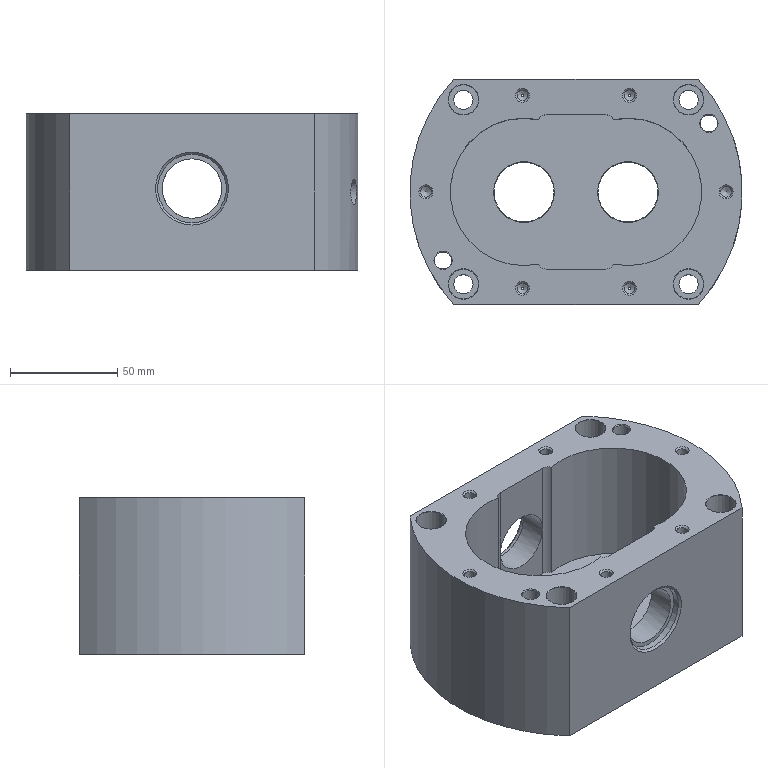NC program | NX | posted with a generic post | part box 155 x 105 x 73.2 mm
Lines 11999 to 12789 of 30727:
(ZLEVEL_PROFILE_COPY_COPY_1 , TOOL : D8)
N23972 T08 M6
N23974 G54
N23976 G17 G0 G90 X-15.89 Y-28.368 B0. C0. S3740 M3
N23978 G43 Z30. H8
N23980 Z-0.1
N23982 G94 G1 X-15.705 Y-29.791 F1000.
N23984 G3 X-15.343 Y-30.362 R0.8
N23986 G2 X-13.894 Y-32. R4. F1600.
N23988 G1 X-10.402
N23990 G3 X-9.789 Y-31.714 R0.8
N23992 G1 X-8.687 Y-30.4
N23994 G0 X-15.89 Y-28.368 Z-0.2
N23996 G1 X-15.705 Y-29.791 F1000.
N23998 G3 X-15.343 Y-30.362 R0.8
N24000 G2 X-13.894 Y-32. R4. F1600.
N24002 G1 X-10.402
N24004 G3 X-9.789 Y-31.714 R0.8
N24006 G1 X-8.687 Y-30.4
N24008 G0 X-15.89 Y-28.368 Z-0.3
N24010 G1 X-15.705 Y-29.791 F1000.
N24012 G3 X-15.343 Y-30.362 R0.8
N24014 G2 X-13.894 Y-32. R4. F1600.
N24016 G1 X-10.402
N24018 G3 X-9.789 Y-31.714 R0.8
N24020 G1 X-8.687 Y-30.4
N24022 G0 X-15.89 Y-28.368 Z-0.4
N24024 G1 X-15.705 Y-29.791 F1000.
N24026 G3 X-15.343 Y-30.362 R0.8
N24028 G2 X-13.894 Y-32. R4. F1600.
N24030 G1 X-10.402
N24032 G3 X-9.789 Y-31.714 R0.8
N24034 G1 X-8.687 Y-30.4
N24036 G0 X-15.89 Y-28.368 Z-0.5
N24038 G1 X-15.705 Y-29.791 F1000.
N24040 G3 X-15.343 Y-30.362 R0.8
N24042 G2 X-13.894 Y-32. R4. F1600.
N24044 G1 X-10.402
N24046 G3 X-9.789 Y-31.714 R0.8
N24048 G1 X-8.687 Y-30.4
N24050 G0 X-15.89 Y-28.368 Z-0.6
N24052 G1 X-15.705 Y-29.791 F1000.
N24054 G3 X-15.343 Y-30.362 R0.8
N24056 G2 X-13.894 Y-32. R4. F1600.
N24058 G1 X-10.402
N24060 G3 X-9.789 Y-31.714 R0.8
N24062 G1 X-8.687 Y-30.4
N24064 G0 X-15.89 Y-28.368 Z-0.7
N24066 G1 X-15.705 Y-29.791 F1000.
N24068 G3 X-15.343 Y-30.362 R0.8
N24070 G2 X-13.894 Y-32. R4. F1600.
N24072 G1 X-10.402
N24074 G3 X-9.789 Y-31.714 R0.8
N24076 G1 X-8.687 Y-30.4
N24078 G0 X-15.89 Y-28.368 Z-0.8
N24080 G1 X-15.705 Y-29.791 F1000.
N24082 G3 X-15.343 Y-30.362 R0.8
N24084 G2 X-13.894 Y-32. R4. F1600.
N24086 G1 X-10.402
N24088 G3 X-9.789 Y-31.714 R0.8
N24090 G1 X-8.687 Y-30.4
N24092 G0 X-15.89 Y-28.368 Z-0.9
N24094 G1 X-15.705 Y-29.791 F1000.
N24096 G3 X-15.343 Y-30.362 R0.8
N24098 G2 X-13.894 Y-32. R4. F1600.
N24100 G1 X-10.402
N24102 G3 X-9.789 Y-31.714 R0.8
N24104 G1 X-8.687 Y-30.4
N24106 G0 X-15.89 Y-28.368 Z-1.
N24108 G1 X-15.705 Y-29.791 F1000.
N24110 G3 X-15.343 Y-30.362 R0.8
N24112 G2 X-13.894 Y-32. R4. F1600.
N24114 G1 X-10.402
N24116 G3 X-9.789 Y-31.714 R0.8
N24118 G1 X-8.687 Y-30.4
N24120 G0 X-15.89 Y-28.368 Z-1.1
N24122 G1 X-15.705 Y-29.791 F1000.
N24124 G3 X-15.343 Y-30.362 R0.8
N24126 G2 X-13.894 Y-32. R4. F1600.
N24128 G1 X-10.402
N24130 G3 X-9.789 Y-31.714 R0.8
N24132 G1 X-8.687 Y-30.4
N24134 G0 X-15.89 Y-28.368 Z-1.2
N24136 G1 X-15.705 Y-29.791 F1000.
N24138 G3 X-15.343 Y-30.362 R0.8
N24140 G2 X-13.894 Y-32. R4. F1600.
N24142 G1 X-10.402
N24144 G3 X-9.789 Y-31.714 R0.8
N24146 G1 X-8.687 Y-30.4
N24148 G0 X-15.89 Y-28.368 Z-1.3
N24150 G1 X-15.705 Y-29.791 F1000.
N24152 G3 X-15.343 Y-30.362 R0.8
N24154 G2 X-13.894 Y-32. R4. F1600.
N24156 G1 X-10.402
N24158 G3 X-9.789 Y-31.714 R0.8
N24160 G1 X-8.687 Y-30.4
N24162 G0 X-15.89 Y-28.368 Z-1.4
N24164 G1 X-15.705 Y-29.791 F1000.
N24166 G3 X-15.343 Y-30.362 R0.8
N24168 G2 X-13.894 Y-32. R4. F1600.
N24170 G1 X-10.402
N24172 G3 X-9.789 Y-31.714 R0.8
N24174 G1 X-8.687 Y-30.4
N24176 G0 X-15.89 Y-28.368 Z-1.5
N24178 G1 X-15.705 Y-29.791 F1000.
N24180 G3 X-15.343 Y-30.362 R0.8
N24182 G2 X-13.894 Y-32. R4. F1600.
N24184 G1 X-10.402
N24186 G3 X-9.789 Y-31.714 R0.8
N24188 G1 X-8.687 Y-30.4
N24190 G0 X-15.89 Y-28.368 Z-1.6
N24192 G1 X-15.705 Y-29.791 F1000.
N24194 G3 X-15.343 Y-30.362 R0.8
N24196 G2 X-13.894 Y-32. R4. F1600.
N24198 G1 X-10.402
N24200 G3 X-9.789 Y-31.714 R0.8
N24202 G1 X-8.687 Y-30.4
N24204 G0 X-15.89 Y-28.368 Z-1.7
N24206 G1 X-15.705 Y-29.791 F1000.
N24208 G3 X-15.343 Y-30.362 R0.8
N24210 G2 X-13.894 Y-32. R4. F1600.
N24212 G1 X-10.402
N24214 G3 X-9.789 Y-31.714 R0.8
N24216 G1 X-8.687 Y-30.4
N24218 G0 X-15.89 Y-28.368 Z-1.8
N24220 G1 X-15.705 Y-29.791 F1000.
N24222 G3 X-15.343 Y-30.362 R0.8
N24224 G2 X-13.894 Y-32. R4. F1600.
N24226 G1 X-10.402
N24228 G3 X-9.789 Y-31.714 R0.8
N24230 G1 X-8.687 Y-30.4
N24232 G0 X-15.89 Y-28.368 Z-1.9
N24234 G1 X-15.705 Y-29.791 F1000.
N24236 G3 X-15.343 Y-30.362 R0.8
N24238 G2 X-13.894 Y-32. R4. F1600.
N24240 G1 X-10.402
N24242 G3 X-9.789 Y-31.714 R0.8
N24244 G1 X-8.687 Y-30.4
N24246 G0 X-15.89 Y-28.368 Z-2.
N24248 G1 X-15.705 Y-29.791 F1000.
N24250 G3 X-15.343 Y-30.362 R0.8
N24252 G2 X-13.894 Y-32. R4. F1600.
N24254 G1 X-10.402
N24256 G3 X-9.789 Y-31.714 R0.8
N24258 G1 X-8.687 Y-30.4
N24260 G0 X-15.89 Y-28.368 Z-2.1
N24262 G1 X-15.705 Y-29.791 F1000.
N24264 G3 X-15.343 Y-30.362 R0.8
N24266 G2 X-13.894 Y-32. R4. F1600.
N24268 G1 X-10.402
N24270 G3 X-9.789 Y-31.714 R0.8
N24272 G1 X-8.687 Y-30.4
N24274 G0 X-15.89 Y-28.368 Z-2.2
N24276 G1 X-15.705 Y-29.791 F1000.
N24278 G3 X-15.343 Y-30.362 R0.8
N24280 G2 X-13.894 Y-32. R4. F1600.
N24282 G1 X-10.402
N24284 G3 X-9.789 Y-31.714 R0.8
N24286 G1 X-8.687 Y-30.4
N24288 G0 X-15.89 Y-28.368 Z-2.3
N24290 G1 X-15.705 Y-29.791 F1000.
N24292 G3 X-15.343 Y-30.362 R0.8
N24294 G2 X-13.894 Y-32. R4. F1600.
N24296 G1 X-10.402
N24298 G3 X-9.789 Y-31.714 R0.8
N24300 G1 X-8.687 Y-30.4
N24302 G0 X-15.89 Y-28.368 Z-2.4
N24304 G1 X-15.705 Y-29.791 F1000.
N24306 G3 X-15.343 Y-30.362 R0.8
N24308 G2 X-13.894 Y-32. R4. F1600.
N24310 G1 X-10.402
N24312 G3 X-9.789 Y-31.714 R0.8
N24314 G1 X-8.687 Y-30.4
N24316 G0 X-15.89 Y-28.368 Z-2.5
N24318 G1 X-15.705 Y-29.791 F1000.
N24320 G3 X-15.343 Y-30.362 R0.8
N24322 G2 X-13.894 Y-32. R4. F1600.
N24324 G1 X-10.402
N24326 G3 X-9.789 Y-31.714 R0.8
N24328 G1 X-8.687 Y-30.4
N24330 G0 X-15.89 Y-28.368 Z-2.6
N24332 G1 X-15.705 Y-29.791 F1000.
N24334 G3 X-15.343 Y-30.362 R0.8
N24336 G2 X-13.894 Y-32. R4. F1600.
N24338 G1 X-10.402
N24340 G3 X-9.789 Y-31.714 R0.8
N24342 G1 X-8.687 Y-30.4
N24344 G0 X-15.89 Y-28.368 Z-2.7
N24346 G1 X-15.705 Y-29.791 F1000.
N24348 G3 X-15.343 Y-30.362 R0.8
N24350 G2 X-13.894 Y-32. R4. F1600.
N24352 G1 X-10.402
N24354 G3 X-9.789 Y-31.714 R0.8
N24356 G1 X-8.687 Y-30.4
N24358 G0 X-15.89 Y-28.368 Z-2.8
N24360 G1 X-15.705 Y-29.791 F1000.
N24362 G3 X-15.343 Y-30.362 R0.8
N24364 G2 X-13.894 Y-32. R4. F1600.
N24366 G1 X-10.402
N24368 G3 X-9.789 Y-31.714 R0.8
N24370 G1 X-8.687 Y-30.4
N24372 G0 X-15.89 Y-28.368 Z-2.9
N24374 G1 X-15.705 Y-29.791 F1000.
N24376 G3 X-15.343 Y-30.362 R0.8
N24378 G2 X-13.894 Y-32. R4. F1600.
N24380 G1 X-10.402
N24382 G3 X-9.789 Y-31.714 R0.8
N24384 G1 X-8.687 Y-30.4
N24386 G0 X-15.89 Y-28.368 Z-3.
N24388 G1 X-15.705 Y-29.791 F1000.
N24390 G3 X-15.343 Y-30.362 R0.8
N24392 G2 X-13.894 Y-32. R4. F1600.
N24394 G1 X-10.402
N24396 G3 X-9.789 Y-31.714 R0.8
N24398 G1 X-8.687 Y-30.4
N24400 G0 X-15.89 Y-28.368 Z-3.1
N24402 G1 X-15.705 Y-29.791 F1000.
N24404 G3 X-15.343 Y-30.362 R0.8
N24406 G2 X-13.894 Y-32. R4. F1600.
N24408 G1 X-10.402
N24410 G3 X-9.789 Y-31.714 R0.8
N24412 G1 X-8.687 Y-30.4
N24414 G0 X-15.89 Y-28.368 Z-3.2
N24416 G1 X-15.705 Y-29.791 F1000.
N24418 G3 X-15.343 Y-30.362 R0.8
N24420 G2 X-13.894 Y-32. R4. F1600.
N24422 G1 X-10.402
N24424 G3 X-9.789 Y-31.714 R0.8
N24426 G1 X-8.687 Y-30.4
N24428 G0 X-15.89 Y-28.368 Z-3.3
N24430 G1 X-15.705 Y-29.791 F1000.
N24432 G3 X-15.343 Y-30.362 R0.8
N24434 G2 X-13.894 Y-32. R4. F1600.
N24436 G1 X-10.402
N24438 G3 X-9.789 Y-31.714 R0.8
N24440 G1 X-8.687 Y-30.4
N24442 G0 X-15.89 Y-28.368 Z-3.4
N24444 G1 X-15.705 Y-29.791 F1000.
N24446 G3 X-15.343 Y-30.362 R0.8
N24448 G2 X-13.894 Y-32. R4. F1600.
N24450 G1 X-10.402
N24452 G3 X-9.789 Y-31.714 R0.8
N24454 G1 X-8.687 Y-30.4
N24456 G0 X-15.89 Y-28.368 Z-3.5
N24458 G1 X-15.705 Y-29.791 F1000.
N24460 G3 X-15.343 Y-30.362 R0.8
N24462 G2 X-13.894 Y-32. R4. F1600.
N24464 G1 X-10.402
N24466 G3 X-9.789 Y-31.714 R0.8
N24468 G1 X-8.687 Y-30.4
N24470 G0 X-15.89 Y-28.368 Z-3.6
N24472 G1 X-15.705 Y-29.791 F1000.
N24474 G3 X-15.343 Y-30.362 R0.8
N24476 G2 X-13.894 Y-32. R4. F1600.
N24478 G1 X-10.402
N24480 G3 X-9.789 Y-31.714 R0.8
N24482 G1 X-8.687 Y-30.4
N24484 G0 X-15.89 Y-28.368 Z-3.7
N24486 G1 X-15.705 Y-29.791 F1000.
N24488 G3 X-15.343 Y-30.362 R0.8
N24490 G2 X-13.894 Y-32. R4. F1600.
N24492 G1 X-10.402
N24494 G3 X-9.789 Y-31.714 R0.8
N24496 G1 X-8.687 Y-30.4
N24498 G0 X-15.89 Y-28.368 Z-3.8
N24500 G1 X-15.705 Y-29.791 F1000.
N24502 G3 X-15.343 Y-30.362 R0.8
N24504 G2 X-13.894 Y-32. R4. F1600.
N24506 G1 X-10.402
N24508 G3 X-9.789 Y-31.714 R0.8
N24510 G1 X-8.687 Y-30.4
N24512 G0 X-15.89 Y-28.368 Z-3.9
N24514 G1 X-15.705 Y-29.791 F1000.
N24516 G3 X-15.343 Y-30.362 R0.8
N24518 G2 X-13.894 Y-32. R4. F1600.
N24520 G1 X-10.402
N24522 G3 X-9.789 Y-31.714 R0.8
N24524 G1 X-8.687 Y-30.4
N24526 G0 X-15.89 Y-28.368 Z-4.
N24528 G1 X-15.705 Y-29.791 F1000.
N24530 G3 X-15.343 Y-30.362 R0.8
N24532 G2 X-13.894 Y-32. R4. F1600.
N24534 G1 X-10.402
N24536 G3 X-9.789 Y-31.714 R0.8
N24538 G1 X-8.687 Y-30.4
N24540 G0 X-15.89 Y-28.368 Z-4.1
N24542 G1 X-15.705 Y-29.791 F1000.
N24544 G3 X-15.343 Y-30.362 R0.8
N24546 G2 X-13.894 Y-32. R4. F1600.
N24548 G1 X-10.402
N24550 G3 X-9.789 Y-31.714 R0.8
N24552 G1 X-8.687 Y-30.4
N24554 G0 X-15.89 Y-28.368 Z-4.2
N24556 G1 X-15.705 Y-29.791 F1000.
N24558 G3 X-15.343 Y-30.362 R0.8
N24560 G2 X-13.894 Y-32. R4. F1600.
N24562 G1 X-10.402
N24564 G3 X-9.789 Y-31.714 R0.8
N24566 G1 X-8.687 Y-30.4
N24568 G0 X-15.89 Y-28.368 Z-4.3
N24570 G1 X-15.705 Y-29.791 F1000.
N24572 G3 X-15.343 Y-30.362 R0.8
N24574 G2 X-13.894 Y-32. R4. F1600.
N24576 G1 X-10.402
N24578 G3 X-9.789 Y-31.714 R0.8
N24580 G1 X-8.687 Y-30.4
N24582 G0 X-15.89 Y-28.368 Z-4.4
N24584 G1 X-15.705 Y-29.791 F1000.
N24586 G3 X-15.343 Y-30.362 R0.8
N24588 G2 X-13.894 Y-32. R4. F1600.
N24590 G1 X-10.402
N24592 G3 X-9.789 Y-31.714 R0.8
N24594 G1 X-8.687 Y-30.4
N24596 G0 X-15.89 Y-28.368 Z-4.5
N24598 G1 X-15.705 Y-29.791 F1000.
N24600 G3 X-15.343 Y-30.362 R0.8
N24602 G2 X-13.894 Y-32. R4. F1600.
N24604 G1 X-10.402
N24606 G3 X-9.789 Y-31.714 R0.8
N24608 G1 X-8.687 Y-30.4
N24610 G0 X-15.89 Y-28.368 Z-4.6
N24612 G1 X-15.705 Y-29.791 F1000.
N24614 G3 X-15.343 Y-30.362 R0.8
N24616 G2 X-13.894 Y-32. R4. F1600.
N24618 G1 X-10.402
N24620 G3 X-9.789 Y-31.714 R0.8
N24622 G1 X-8.687 Y-30.4
N24624 G0 X-15.89 Y-28.368 Z-4.7
N24626 G1 X-15.705 Y-29.791 F1000.
N24628 G3 X-15.343 Y-30.362 R0.8
N24630 G2 X-13.894 Y-32. R4. F1600.
N24632 G1 X-10.402
N24634 G3 X-9.789 Y-31.714 R0.8
N24636 G1 X-8.687 Y-30.4
N24638 G0 X-15.89 Y-28.368 Z-4.8
N24640 G1 X-15.705 Y-29.791 F1000.
N24642 G3 X-15.343 Y-30.362 R0.8
N24644 G2 X-13.894 Y-32. R4. F1600.
N24646 G1 X-10.402
N24648 G3 X-9.789 Y-31.714 R0.8
N24650 G1 X-8.687 Y-30.4
N24652 G0 X-15.89 Y-28.368 Z-4.9
N24654 G1 X-15.705 Y-29.791 F1000.
N24656 G3 X-15.343 Y-30.362 R0.8
N24658 G2 X-13.894 Y-32. R4. F1600.
N24660 G1 X-10.402
N24662 G3 X-9.789 Y-31.714 R0.8
N24664 G1 X-8.687 Y-30.4
N24666 G0 X-15.89 Y-28.368 Z-5.
N24668 G1 X-15.705 Y-29.791 F1000.
N24670 G3 X-15.343 Y-30.362 R0.8
N24672 G2 X-13.894 Y-32. R4. F1600.
N24674 G1 X-10.402
N24676 G3 X-9.789 Y-31.714 R0.8
N24678 G1 X-8.687 Y-30.4
N24680 G0 X-15.89 Y-28.368 Z-5.1
N24682 G1 X-15.705 Y-29.791 F1000.
N24684 G3 X-15.343 Y-30.362 R0.8
N24686 G2 X-13.894 Y-32. R4. F1600.
N24688 G1 X-10.402
N24690 G3 X-9.789 Y-31.714 R0.8
N24692 G1 X-8.687 Y-30.4
N24694 G0 X-15.89 Y-28.368 Z-5.2
N24696 G1 X-15.705 Y-29.791 F1000.
N24698 G3 X-15.343 Y-30.362 R0.8
N24700 G2 X-13.894 Y-32. R4. F1600.
N24702 G1 X-10.402
N24704 G3 X-9.789 Y-31.714 R0.8
N24706 G1 X-8.687 Y-30.4
N24708 G0 X-15.89 Y-28.368 Z-5.3
N24710 G1 X-15.705 Y-29.791 F1000.
N24712 G3 X-15.343 Y-30.362 R0.8
N24714 G2 X-13.894 Y-32. R4. F1600.
N24716 G1 X-10.402
N24718 G3 X-9.789 Y-31.714 R0.8
N24720 G1 X-8.687 Y-30.4
N24722 G0 X-15.89 Y-28.368 Z-5.4
N24724 G1 X-15.705 Y-29.791 F1000.
N24726 G3 X-15.343 Y-30.362 R0.8
N24728 G2 X-13.894 Y-32. R4. F1600.
N24730 G1 X-10.402
N24732 G3 X-9.789 Y-31.714 R0.8
N24734 G1 X-8.687 Y-30.4
N24736 G0 X-15.89 Y-28.368 Z-5.5
N24738 G1 X-15.705 Y-29.791 F1000.
N24740 G3 X-15.343 Y-30.362 R0.8
N24742 G2 X-13.894 Y-32. R4. F1600.
N24744 G1 X-10.402
N24746 G3 X-9.789 Y-31.714 R0.8
N24748 G1 X-8.687 Y-30.4
N24750 G0 X-15.89 Y-28.368 Z-5.6
N24752 G1 X-15.705 Y-29.791 F1000.
N24754 G3 X-15.343 Y-30.362 R0.8
N24756 G2 X-13.894 Y-32. R4. F1600.
N24758 G1 X-10.402
N24760 G3 X-9.789 Y-31.714 R0.8
N24762 G1 X-8.687 Y-30.4
N24764 G0 X-15.89 Y-28.368 Z-5.7
N24766 G1 X-15.705 Y-29.791 F1000.
N24768 G3 X-15.343 Y-30.362 R0.8
N24770 G2 X-13.894 Y-32. R4. F1600.
N24772 G1 X-10.402
N24774 G3 X-9.789 Y-31.714 R0.8
N24776 G1 X-8.687 Y-30.4
N24778 G0 X-15.89 Y-28.368 Z-5.8
N24780 G1 X-15.705 Y-29.791 F1000.
N24782 G3 X-15.343 Y-30.362 R0.8
N24784 G2 X-13.894 Y-32. R4. F1600.
N24786 G1 X-10.402
N24788 G3 X-9.789 Y-31.714 R0.8
N24790 G1 X-8.687 Y-30.4
N24792 G0 X-15.89 Y-28.368 Z-5.9
N24794 G1 X-15.705 Y-29.791 F1000.
N24796 G3 X-15.343 Y-30.362 R0.8
N24798 G2 X-13.894 Y-32. R4. F1600.
N24800 G1 X-10.402
N24802 G3 X-9.789 Y-31.714 R0.8
N24804 G1 X-8.687 Y-30.4
N24806 G0 X-15.89 Y-28.368 Z-6.
N24808 G1 X-15.705 Y-29.791 F1000.
N24810 G3 X-15.343 Y-30.362 R0.8
N24812 G2 X-13.894 Y-32. R4. F1600.
N24814 G1 X-10.402
N24816 G3 X-9.789 Y-31.714 R0.8
N24818 G1 X-8.687 Y-30.4
N24820 G0 X-15.89 Y-28.368 Z-6.1
N24822 G1 X-15.705 Y-29.791 F1000.
N24824 G3 X-15.343 Y-30.362 R0.8
N24826 G2 X-13.894 Y-32. R4. F1600.
N24828 G1 X-10.402
N24830 G3 X-9.789 Y-31.714 R0.8
N24832 G1 X-8.687 Y-30.4
N24834 G0 X-15.89 Y-28.368 Z-6.2
N24836 G1 X-15.705 Y-29.791 F1000.
N24838 G3 X-15.343 Y-30.362 R0.8
N24840 G2 X-13.894 Y-32. R4. F1600.
N24842 G1 X-10.402
N24844 G3 X-9.789 Y-31.714 R0.8
N24846 G1 X-8.687 Y-30.4
N24848 G0 X-15.89 Y-28.368 Z-6.3
N24850 G1 X-15.705 Y-29.791 F1000.
N24852 G3 X-15.343 Y-30.362 R0.8
N24854 G2 X-13.894 Y-32. R4. F1600.
N24856 G1 X-10.402
N24858 G3 X-9.789 Y-31.714 R0.8
N24860 G1 X-8.687 Y-30.4
N24862 G0 X-15.89 Y-28.368 Z-6.4
N24864 G1 X-15.705 Y-29.791 F1000.
N24866 G3 X-15.343 Y-30.362 R0.8
N24868 G2 X-13.894 Y-32. R4. F1600.
N24870 G1 X-10.402
N24872 G3 X-9.789 Y-31.714 R0.8
N24874 G1 X-8.687 Y-30.4
N24876 G0 X-15.89 Y-28.368 Z-6.5
N24878 G1 X-15.705 Y-29.791 F1000.
N24880 G3 X-15.343 Y-30.362 R0.8
N24882 G2 X-13.894 Y-32. R4. F1600.
N24884 G1 X-10.402
N24886 G3 X-9.789 Y-31.714 R0.8
N24888 G1 X-8.687 Y-30.4
N24890 G0 X-15.89 Y-28.368 Z-6.6
N24892 G1 X-15.705 Y-29.791 F1000.
N24894 G3 X-15.343 Y-30.362 R0.8
N24896 G2 X-13.894 Y-32. R4. F1600.
N24898 G1 X-10.402
N24900 G3 X-9.789 Y-31.714 R0.8
N24902 G1 X-8.687 Y-30.4
N24904 G0 X-15.89 Y-28.368 Z-6.7
N24906 G1 X-15.705 Y-29.791 F1000.
N24908 G3 X-15.343 Y-30.362 R0.8
N24910 G2 X-13.894 Y-32. R4. F1600.
N24912 G1 X-10.402
N24914 G3 X-9.789 Y-31.714 R0.8
N24916 G1 X-8.687 Y-30.4
N24918 G0 X-15.89 Y-28.368 Z-6.8
N24920 G1 X-15.705 Y-29.791 F1000.
N24922 G3 X-15.343 Y-30.362 R0.8
N24924 G2 X-13.894 Y-32. R4. F1600.
N24926 G1 X-10.402
N24928 G3 X-9.789 Y-31.714 R0.8
N24930 G1 X-8.687 Y-30.4
N24932 G0 X-15.89 Y-28.368 Z-6.9
N24934 G1 X-15.705 Y-29.791 F1000.
N24936 G3 X-15.343 Y-30.362 R0.8
N24938 G2 X-13.894 Y-32. R4. F1600.
N24940 G1 X-10.402
N24942 G3 X-9.789 Y-31.714 R0.8
N24944 G1 X-8.687 Y-30.4
N24946 G0 X-15.89 Y-28.368 Z-7.
N24948 G1 X-15.705 Y-29.791 F1000.
N24950 G3 X-15.343 Y-30.362 R0.8
N24952 G2 X-13.894 Y-32. R4. F1600.
N24954 G1 X-10.402
N24956 G3 X-9.789 Y-31.714 R0.8
N24958 G1 X-8.687 Y-30.4
N24960 G0 X-15.89 Y-28.368 Z-7.1
N24962 G1 X-15.705 Y-29.791 F1000.
N24964 G3 X-15.343 Y-30.362 R0.8
N24966 G2 X-13.894 Y-32. R4. F1600.
N24968 G1 X-10.402
N24970 G3 X-9.789 Y-31.714 R0.8
N24972 G1 X-8.687 Y-30.4
N24974 G0 X-15.89 Y-28.368 Z-7.2
N24976 G1 X-15.705 Y-29.791 F1000.
N24978 G3 X-15.343 Y-30.362 R0.8
N24980 G2 X-13.894 Y-32. R4. F1600.
N24982 G1 X-10.402
N24984 G3 X-9.789 Y-31.714 R0.8
N24986 G1 X-8.687 Y-30.4
N24988 G0 X-15.89 Y-28.368 Z-7.3
N24990 G1 X-15.705 Y-29.791 F1000.
N24992 G3 X-15.343 Y-30.362 R0.8
N24994 G2 X-13.894 Y-32. R4. F1600.
N24996 G1 X-10.402
N24998 G3 X-9.789 Y-31.714 R0.8
N25000 G1 X-8.687 Y-30.4
N25002 G0 X-15.89 Y-28.368 Z-7.4
N25004 G1 X-15.705 Y-29.791 F1000.
N25006 G3 X-15.343 Y-30.362 R0.8
N25008 G2 X-13.894 Y-32. R4. F1600.
N25010 G1 X-10.402
N25012 G3 X-9.789 Y-31.714 R0.8
N25014 G1 X-8.687 Y-30.4
N25016 G0 X-15.89 Y-28.368 Z-7.5
N25018 G1 X-15.705 Y-29.791 F1000.
N25020 G3 X-15.343 Y-30.362 R0.8
N25022 G2 X-13.894 Y-32. R4. F1600.
N25024 G1 X-10.402
N25026 G3 X-9.789 Y-31.714 R0.8
N25028 G1 X-8.687 Y-30.4
N25030 G0 X-15.89 Y-28.368 Z-7.6
N25032 G1 X-15.705 Y-29.791 F1000.
N25034 G3 X-15.343 Y-30.362 R0.8
N25036 G2 X-13.894 Y-32. R4. F1600.
N25038 G1 X-10.402
N25040 G3 X-9.789 Y-31.714 R0.8
N25042 G1 X-8.687 Y-30.4
N25044 G0 X-15.89 Y-28.368 Z-7.7
N25046 G1 X-15.705 Y-29.791 F1000.
N25048 G3 X-15.343 Y-30.362 R0.8
N25050 G2 X-13.894 Y-32. R4. F1600.
N25052 G1 X-10.402
N25054 G3 X-9.789 Y-31.714 R0.8
N25056 G1 X-8.687 Y-30.4
N25058 G0 X-15.89 Y-28.368 Z-7.8
N25060 G1 X-15.705 Y-29.791 F1000.
N25062 G3 X-15.343 Y-30.362 R0.8
N25064 G2 X-13.894 Y-32. R4. F1600.
N25066 G1 X-10.402
N25068 G3 X-9.789 Y-31.714 R0.8
N25070 G1 X-8.687 Y-30.4
N25072 G0 X-15.89 Y-28.368 Z-7.9
N25074 G1 X-15.705 Y-29.791 F1000.
N25076 G3 X-15.343 Y-30.362 R0.8
N25078 G2 X-13.894 Y-32. R4. F1600.
N25080 G1 X-10.402
N25082 G3 X-9.789 Y-31.714 R0.8
N25084 G1 X-8.687 Y-30.4
N25086 G0 X-15.89 Y-28.368 Z-8.
N25088 G1 X-15.705 Y-29.791 F1000.
N25090 G3 X-15.343 Y-30.362 R0.8
N25092 G2 X-13.894 Y-32. R4. F1600.
N25094 G1 X-10.402
N25096 G3 X-9.789 Y-31.714 R0.8
N25098 G1 X-8.687 Y-30.4
N25100 G0 X-15.89 Y-28.368 Z-8.1
N25102 G1 X-15.705 Y-29.791 F1000.
N25104 G3 X-15.343 Y-30.362 R0.8
N25106 G2 X-13.894 Y-32. R4. F1600.
N25108 G1 X-10.402
N25110 G3 X-9.789 Y-31.714 R0.8
N25112 G1 X-8.687 Y-30.4
N25114 G0 X-15.89 Y-28.368 Z-8.2
N25116 G1 X-15.705 Y-29.791 F1000.
N25118 G3 X-15.343 Y-30.362 R0.8
N25120 G2 X-13.894 Y-32. R4. F1600.
N25122 G1 X-10.402
N25124 G3 X-9.789 Y-31.714 R0.8
N25126 G1 X-8.687 Y-30.4
N25128 G0 X-15.89 Y-28.368 Z-8.3
N25130 G1 X-15.705 Y-29.791 F1000.
N25132 G3 X-15.343 Y-30.362 R0.8
N25134 G2 X-13.894 Y-32. R4. F1600.
N25136 G1 X-10.402
N25138 G3 X-9.789 Y-31.714 R0.8
N25140 G1 X-8.687 Y-30.4
N25142 G0 X-15.89 Y-28.368 Z-8.4
N25144 G1 X-15.705 Y-29.791 F1000.
N25146 G3 X-15.343 Y-30.362 R0.8
N25148 G2 X-13.894 Y-32. R4. F1600.
N25150 G1 X-10.402
N25152 G3 X-9.789 Y-31.714 R0.8
N25154 G1 X-8.687 Y-30.4
N25156 G0 X-15.89 Y-28.368 Z-8.5
N25158 G1 X-15.705 Y-29.791 F1000.
N25160 G3 X-15.343 Y-30.362 R0.8
N25162 G2 X-13.894 Y-32. R4. F1600.
N25164 G1 X-10.402
N25166 G3 X-9.789 Y-31.714 R0.8
N25168 G1 X-8.687 Y-30.4
N25170 G0 X-15.89 Y-28.368 Z-8.6
N25172 G1 X-15.705 Y-29.791 F1000.
N25174 G3 X-15.343 Y-30.362 R0.8
N25176 G2 X-13.894 Y-32. R4. F1600.
N25178 G1 X-10.402
N25180 G3 X-9.789 Y-31.714 R0.8
N25182 G1 X-8.687 Y-30.4
N25184 G0 X-15.89 Y-28.368 Z-8.7
N25186 G1 X-15.705 Y-29.791 F1000.
N25188 G3 X-15.343 Y-30.362 R0.8
N25190 G2 X-13.894 Y-32. R4. F1600.
N25192 G1 X-10.402
N25194 G3 X-9.789 Y-31.714 R0.8
N25196 G1 X-8.687 Y-30.4
N25198 G0 X-15.89 Y-28.368 Z-8.8
N25200 G1 X-15.705 Y-29.791 F1000.
N25202 G3 X-15.343 Y-30.362 R0.8
N25204 G2 X-13.894 Y-32. R4. F1600.
N25206 G1 X-10.402
N25208 G3 X-9.789 Y-31.714 R0.8
N25210 G1 X-8.687 Y-30.4
N25212 G0 X-15.89 Y-28.368 Z-8.9
N25214 G1 X-15.705 Y-29.791 F1000.
N25216 G3 X-15.343 Y-30.362 R0.8
N25218 G2 X-13.894 Y-32. R4. F1600.
N25220 G1 X-10.402
N25222 G3 X-9.789 Y-31.714 R0.8
N25224 G1 X-8.687 Y-30.4
N25226 G0 X-15.89 Y-28.368 Z-9.
N25228 G1 X-15.705 Y-29.791 F1000.
N25230 G3 X-15.343 Y-30.362 R0.8
N25232 G2 X-13.894 Y-32. R4. F1600.
N25234 G1 X-10.402
N25236 G3 X-9.789 Y-31.714 R0.8
N25238 G1 X-8.687 Y-30.4
N25240 G0 X-15.89 Y-28.368 Z-9.1
N25242 G1 X-15.705 Y-29.791 F1000.
N25244 G3 X-15.343 Y-30.362 R0.8
N25246 G2 X-13.894 Y-32. R4. F1600.
N25248 G1 X-10.402
N25250 G3 X-9.789 Y-31.714 R0.8
N25252 G1 X-8.687 Y-30.4
N25254 G0 X-15.89 Y-28.368 Z-9.2
N25256 G1 X-15.705 Y-29.791 F1000.
N25258 G3 X-15.343 Y-30.362 R0.8
N25260 G2 X-13.894 Y-32. R4. F1600.
N25262 G1 X-10.402
N25264 G3 X-9.789 Y-31.714 R0.8
N25266 G1 X-8.687 Y-30.4
N25268 G0 X-15.89 Y-28.368 Z-9.3
N25270 G1 X-15.705 Y-29.791 F1000.
N25272 G3 X-15.343 Y-30.362 R0.8
N25274 G2 X-13.894 Y-32. R4. F1600.
N25276 G1 X-10.402
N25278 G3 X-9.789 Y-31.714 R0.8
N25280 G1 X-8.687 Y-30.4
N25282 G0 X-15.89 Y-28.368 Z-9.4
N25284 G1 X-15.705 Y-29.791 F1000.
N25286 G3 X-15.343 Y-30.362 R0.8
N25288 G2 X-13.894 Y-32. R4. F1600.
N25290 G1 X-10.402
N25292 G3 X-9.789 Y-31.714 R0.8
N25294 G1 X-8.687 Y-30.4
N25296 G0 X-15.89 Y-28.368 Z-9.5
N25298 G1 X-15.705 Y-29.791 F1000.
N25300 G3 X-15.343 Y-30.362 R0.8
N25302 G2 X-13.894 Y-32. R4. F1600.
N25304 G1 X-10.402
N25306 G3 X-9.789 Y-31.714 R0.8
N25308 G1 X-8.687 Y-30.4
N25310 G0 X-15.89 Y-28.368 Z-9.6
N25312 G1 X-15.705 Y-29.791 F1000.
N25314 G3 X-15.343 Y-30.362 R0.8
N25316 G2 X-13.894 Y-32. R4. F1600.
N25318 G1 X-10.402
N25320 G3 X-9.789 Y-31.714 R0.8
N25322 G1 X-8.687 Y-30.4
N25324 G0 X-15.89 Y-28.368 Z-9.7
N25326 G1 X-15.705 Y-29.791 F1000.
N25328 G3 X-15.343 Y-30.362 R0.8
N25330 G2 X-13.894 Y-32. R4. F1600.
N25332 G1 X-10.402
N25334 G3 X-9.789 Y-31.714 R0.8
N25336 G1 X-8.687 Y-30.4
N25338 G0 X-15.89 Y-28.368 Z-9.8
N25340 G1 X-15.705 Y-29.791 F1000.
N25342 G3 X-15.343 Y-30.362 R0.8
N25344 G2 X-13.894 Y-32. R4. F1600.
N25346 G1 X-10.402
N25348 G3 X-9.789 Y-31.714 R0.8
N25350 G1 X-8.687 Y-30.4
N25352 G0 X-15.89 Y-28.368 Z-9.9
N25354 G1 X-15.705 Y-29.791 F1000.
N25356 G3 X-15.343 Y-30.362 R0.8
N25358 G2 X-13.894 Y-32. R4. F1600.
N25360 G1 X-10.402
N25362 G3 X-9.789 Y-31.714 R0.8
N25364 G1 X-8.687 Y-30.4
N25366 G0 X-15.89 Y-28.368 Z-10.
N25368 G1 X-15.705 Y-29.791 F1000.
N25370 G3 X-15.343 Y-30.362 R0.8
N25372 G2 X-13.894 Y-32. R4. F1600.
N25374 G1 X-10.402
N25376 G3 X-9.789 Y-31.714 R0.8
N25378 G1 X-8.687 Y-30.4
N25380 G0 X-15.89 Y-28.368 Z-10.1
N25382 G1 X-15.705 Y-29.791 F1000.
N25384 G3 X-15.343 Y-30.362 R0.8
N25386 G2 X-13.894 Y-32. R4. F1600.
N25388 G1 X-10.402
N25390 G3 X-9.789 Y-31.714 R0.8
N25392 G1 X-8.687 Y-30.4
N25394 G0 X-15.89 Y-28.368 Z-10.2
N25396 G1 X-15.705 Y-29.791 F1000.
N25398 G3 X-15.343 Y-30.362 R0.8
N25400 G2 X-13.894 Y-32. R4. F1600.
N25402 G1 X-10.402
N25404 G3 X-9.789 Y-31.714 R0.8
N25406 G1 X-8.687 Y-30.4
N25408 G0 X-15.89 Y-28.368 Z-10.3
N25410 G1 X-15.705 Y-29.791 F1000.
N25412 G3 X-15.343 Y-30.362 R0.8
N25414 G2 X-13.894 Y-32. R4. F1600.
N25416 G1 X-10.402
N25418 G3 X-9.789 Y-31.714 R0.8
N25420 G1 X-8.687 Y-30.4
N25422 G0 X-15.89 Y-28.368 Z-10.4
N25424 G1 X-15.705 Y-29.791 F1000.
N25426 G3 X-15.343 Y-30.362 R0.8
N25428 G2 X-13.894 Y-32. R4. F1600.
N25430 G1 X-10.402
N25432 G3 X-9.789 Y-31.714 R0.8
N25434 G1 X-8.687 Y-30.4
N25436 G0 X-15.89 Y-28.368 Z-10.5
N25438 G1 X-15.705 Y-29.791 F1000.
N25440 G3 X-15.343 Y-30.362 R0.8
N25442 G2 X-13.894 Y-32. R4. F1600.
N25444 G1 X-10.402
N25446 G3 X-9.789 Y-31.714 R0.8
N25448 G1 X-8.687 Y-30.4
N25450 G0 X-15.89 Y-28.368 Z-10.6
N25452 G1 X-15.705 Y-29.791 F1000.
N25454 G3 X-15.343 Y-30.362 R0.8
N25456 G2 X-13.894 Y-32. R4. F1600.
N25458 G1 X-10.402
N25460 G3 X-9.789 Y-31.714 R0.8
N25462 G1 X-8.687 Y-30.4
N25464 G0 X-15.89 Y-28.368 Z-10.7
N25466 G1 X-15.705 Y-29.791 F1000.
N25468 G3 X-15.343 Y-30.362 R0.8
N25470 G2 X-13.894 Y-32. R4. F1600.
N25472 G1 X-10.402
N25474 G3 X-9.789 Y-31.714 R0.8
N25476 G1 X-8.687 Y-30.4
N25478 G0 X-15.89 Y-28.368 Z-10.8
N25480 G1 X-15.705 Y-29.791 F1000.
N25482 G3 X-15.343 Y-30.362 R0.8
N25484 G2 X-13.894 Y-32. R4. F1600.
N25486 G1 X-10.402
N25488 G3 X-9.789 Y-31.714 R0.8
N25490 G1 X-8.687 Y-30.4
N25492 G0 X-15.89 Y-28.368 Z-10.9
N25494 G1 X-15.705 Y-29.791 F1000.
N25496 G3 X-15.343 Y-30.362 R0.8
N25498 G2 X-13.894 Y-32. R4. F1600.
N25500 G1 X-10.402
N25502 G3 X-9.789 Y-31.714 R0.8
N25504 G1 X-8.687 Y-30.4
N25506 G0 X-15.89 Y-28.368 Z-11.
N25508 G1 X-15.705 Y-29.791 F1000.
N25510 G3 X-15.343 Y-30.362 R0.8
N25512 G2 X-13.894 Y-32. R4. F1600.
N25514 G1 X-10.402
N25516 G3 X-9.789 Y-31.714 R0.8
N25518 G1 X-8.687 Y-30.4
N25520 G0 X-15.89 Y-28.368 Z-11.1
N25522 G1 X-15.705 Y-29.791 F1000.
N25524 G3 X-15.343 Y-30.362 R0.8
N25526 G2 X-13.894 Y-32. R4. F1600.
N25528 G1 X-10.402
N25530 G3 X-9.789 Y-31.714 R0.8
N25532 G1 X-8.687 Y-30.4
N25534 G0 X-15.89 Y-28.368 Z-11.2
N25536 G1 X-15.705 Y-29.791 F1000.
N25538 G3 X-15.343 Y-30.362 R0.8
N25540 G2 X-13.894 Y-32. R4. F1600.
N25542 G1 X-10.402
N25544 G3 X-9.789 Y-31.714 R0.8
N25546 G1 X-8.687 Y-30.4